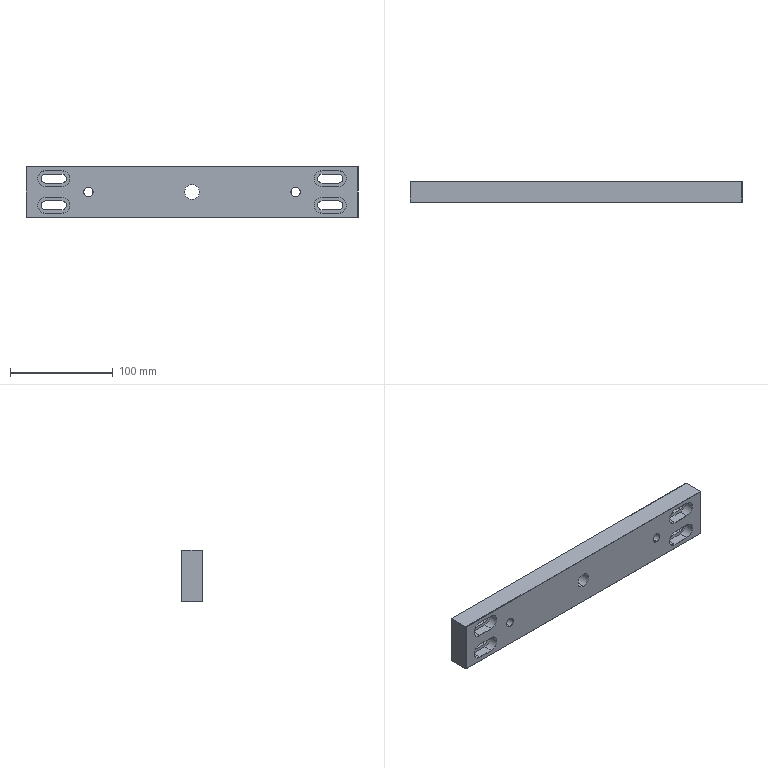Part | 1 solid | 114 faces | box 323 x 20 x 50 mm | volume 291461 mm3 | plane 64 | cylinder 26 | cone 24 | commonest cylinder face diameters 15 x12 8.6 x8 9 x4 14.5 x2